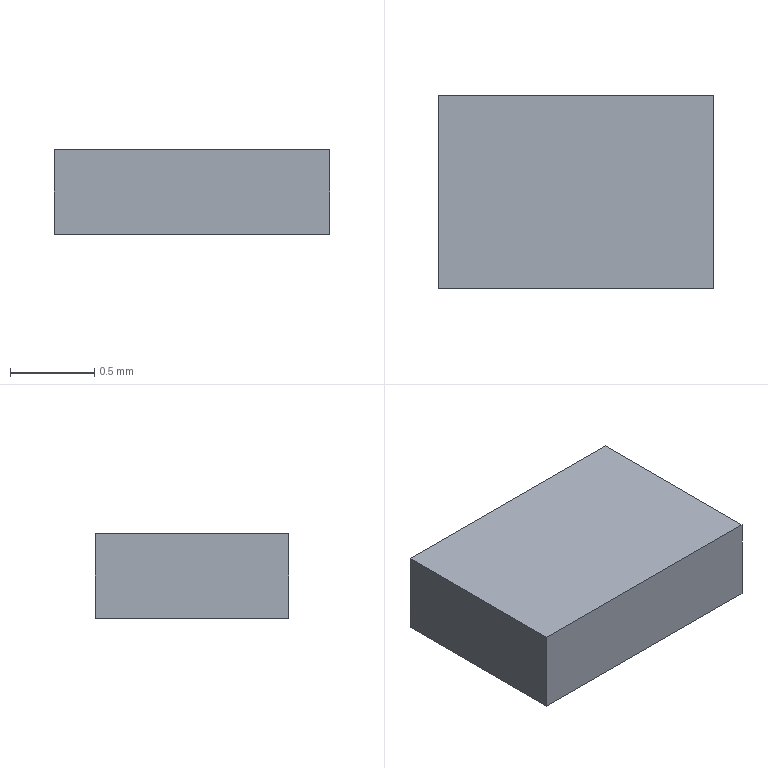Part | Creo | 1 solid | 6 faces | box 1.64 x 1.15 x 0.5 mm | volume 0.9427 mm3 | plane 6
STEP:
#1=CARTESIAN_POINT('',(0.,0.,0.));
#2=DIRECTION('',(0.,0.,1.));
#3=DIRECTION('',(1.,0.,0.));
#4=AXIS2_PLACEMENT_3D('',#1,#2,#3);
#5=CARTESIAN_POINT('',(-0.9145,-0.575,0.));
#6=VERTEX_POINT('',#5);
#7=CARTESIAN_POINT('',(0.725,-0.575,0.));
#8=VERTEX_POINT('',#7);
#9=CARTESIAN_POINT('',(-0.9145,-0.575,0.));
#10=DIRECTION('',(1.,0.,0.));
#11=VECTOR('',#10,1.64);
#12=LINE('',#9,#11);
#13=EDGE_CURVE('',#6,#8,#12,.T.);
#14=ORIENTED_EDGE('',*,*,#13,.T.);
#15=CARTESIAN_POINT('',(0.725,0.575,0.));
#16=VERTEX_POINT('',#15);
#17=CARTESIAN_POINT('',(0.725,-0.575,0.));
#18=DIRECTION('',(0.,1.,0.));
#19=VECTOR('',#18,1.15);
#20=LINE('',#17,#19);
#21=EDGE_CURVE('',#8,#16,#20,.T.);
#22=ORIENTED_EDGE('',*,*,#21,.T.);
#23=CARTESIAN_POINT('',(-0.9145,0.575,0.));
#24=VERTEX_POINT('',#23);
#25=CARTESIAN_POINT('',(0.725,0.575,0.));
#26=DIRECTION('',(-1.,0.,0.));
#27=VECTOR('',#26,1.64);
#28=LINE('',#25,#27);
#29=EDGE_CURVE('',#16,#24,#28,.T.);
#30=ORIENTED_EDGE('',*,*,#29,.T.);
#31=CARTESIAN_POINT('',(-0.9145,0.575,0.));
#32=DIRECTION('',(0.,-1.,0.));
#33=VECTOR('',#32,1.15);
#34=LINE('',#31,#33);
#35=EDGE_CURVE('',#24,#6,#34,.T.);
#36=ORIENTED_EDGE('',*,*,#35,.T.);
#37=EDGE_LOOP('',(#14,#22,#30,#36));
#38=FACE_OUTER_BOUND('',#37,.F.);
#39=CARTESIAN_POINT('',(0.,0.,0.));
#40=DIRECTION('',(0.,0.,1.));
#41=DIRECTION('',(1.,0.,0.));
#42=AXIS2_PLACEMENT_3D('',#39,#40,#41);
#43=PLANE('',#42);
#44=ADVANCED_FACE('',(#38),#43,.F.);
#45=ORIENTED_EDGE('',*,*,#13,.F.);
#46=CARTESIAN_POINT('',(-0.9145,-0.575,0.5));
#47=VERTEX_POINT('',#46);
#48=CARTESIAN_POINT('',(-0.9145,-0.575,0.));
#49=DIRECTION('',(0.,0.,1.));
#50=VECTOR('',#49,0.5);
#51=LINE('',#48,#50);
#52=EDGE_CURVE('',#6,#47,#51,.T.);
#53=ORIENTED_EDGE('',*,*,#52,.T.);
#54=CARTESIAN_POINT('',(0.725,-0.575,0.5));
#55=VERTEX_POINT('',#54);
#56=CARTESIAN_POINT('',(-0.9145,-0.575,0.5));
#57=DIRECTION('',(1.,0.,0.));
#58=VECTOR('',#57,1.64);
#59=LINE('',#56,#58);
#60=EDGE_CURVE('',#47,#55,#59,.T.);
#61=ORIENTED_EDGE('',*,*,#60,.T.);
#62=CARTESIAN_POINT('',(0.725,-0.575,0.));
#63=DIRECTION('',(0.,0.,1.));
#64=VECTOR('',#63,0.5);
#65=LINE('',#62,#64);
#66=EDGE_CURVE('',#8,#55,#65,.T.);
#67=ORIENTED_EDGE('',*,*,#66,.F.);
#68=EDGE_LOOP('',(#45,#53,#61,#67));
#69=FACE_OUTER_BOUND('',#68,.F.);
#70=CARTESIAN_POINT('',(-0.9145,-0.575,0.));
#71=DIRECTION('',(0.,-1.,0.));
#72=DIRECTION('',(1.,0.,0.));
#73=AXIS2_PLACEMENT_3D('',#70,#71,#72);
#74=PLANE('',#73);
#75=ADVANCED_FACE('',(#69),#74,.T.);
#76=ORIENTED_EDGE('',*,*,#35,.F.);
#77=CARTESIAN_POINT('',(-0.9145,0.575,0.5));
#78=VERTEX_POINT('',#77);
#79=CARTESIAN_POINT('',(-0.9145,0.575,0.));
#80=DIRECTION('',(0.,0.,1.));
#81=VECTOR('',#80,0.5);
#82=LINE('',#79,#81);
#83=EDGE_CURVE('',#24,#78,#82,.T.);
#84=ORIENTED_EDGE('',*,*,#83,.T.);
#85=CARTESIAN_POINT('',(-0.9145,0.575,0.5));
#86=DIRECTION('',(0.,-1.,0.));
#87=VECTOR('',#86,1.15);
#88=LINE('',#85,#87);
#89=EDGE_CURVE('',#78,#47,#88,.T.);
#90=ORIENTED_EDGE('',*,*,#89,.T.);
#91=ORIENTED_EDGE('',*,*,#52,.F.);
#92=EDGE_LOOP('',(#76,#84,#90,#91));
#93=FACE_OUTER_BOUND('',#92,.F.);
#94=CARTESIAN_POINT('',(-0.9145,0.575,0.));
#95=DIRECTION('',(-1.,0.,0.));
#96=DIRECTION('',(0.,-1.,0.));
#97=AXIS2_PLACEMENT_3D('',#94,#95,#96);
#98=PLANE('',#97);
#99=ADVANCED_FACE('',(#93),#98,.T.);
#100=ORIENTED_EDGE('',*,*,#29,.F.);
#101=CARTESIAN_POINT('',(0.725,0.575,0.5));
#102=VERTEX_POINT('',#101);
#103=CARTESIAN_POINT('',(0.725,0.575,0.));
#104=DIRECTION('',(0.,0.,1.));
#105=VECTOR('',#104,0.5);
#106=LINE('',#103,#105);
#107=EDGE_CURVE('',#16,#102,#106,.T.);
#108=ORIENTED_EDGE('',*,*,#107,.T.);
#109=CARTESIAN_POINT('',(0.725,0.575,0.5));
#110=DIRECTION('',(-1.,0.,0.));
#111=VECTOR('',#110,1.64);
#112=LINE('',#109,#111);
#113=EDGE_CURVE('',#102,#78,#112,.T.);
#114=ORIENTED_EDGE('',*,*,#113,.T.);
#115=ORIENTED_EDGE('',*,*,#83,.F.);
#116=EDGE_LOOP('',(#100,#108,#114,#115));
#117=FACE_OUTER_BOUND('',#116,.F.);
#118=CARTESIAN_POINT('',(0.725,0.575,0.));
#119=DIRECTION('',(0.,1.,0.));
#120=DIRECTION('',(-1.,0.,0.));
#121=AXIS2_PLACEMENT_3D('',#118,#119,#120);
#122=PLANE('',#121);
#123=ADVANCED_FACE('',(#117),#122,.T.);
#124=ORIENTED_EDGE('',*,*,#21,.F.);
#125=ORIENTED_EDGE('',*,*,#66,.T.);
#126=CARTESIAN_POINT('',(0.725,-0.575,0.5));
#127=DIRECTION('',(0.,1.,0.));
#128=VECTOR('',#127,1.15);
#129=LINE('',#126,#128);
#130=EDGE_CURVE('',#55,#102,#129,.T.);
#131=ORIENTED_EDGE('',*,*,#130,.T.);
#132=ORIENTED_EDGE('',*,*,#107,.F.);
#133=EDGE_LOOP('',(#124,#125,#131,#132));
#134=FACE_OUTER_BOUND('',#133,.F.);
#135=CARTESIAN_POINT('',(0.725,-0.575,0.));
#136=DIRECTION('',(1.,0.,0.));
#137=DIRECTION('',(0.,1.,0.));
#138=AXIS2_PLACEMENT_3D('',#135,#136,#137);
#139=PLANE('',#138);
#140=ADVANCED_FACE('',(#134),#139,.T.);
#141=ORIENTED_EDGE('',*,*,#60,.F.);
#142=ORIENTED_EDGE('',*,*,#89,.F.);
#143=ORIENTED_EDGE('',*,*,#113,.F.);
#144=ORIENTED_EDGE('',*,*,#130,.F.);
#145=EDGE_LOOP('',(#141,#142,#143,#144));
#146=FACE_OUTER_BOUND('',#145,.F.);
#147=CARTESIAN_POINT('',(0.,0.,0.5));
#148=DIRECTION('',(0.,0.,1.));
#149=DIRECTION('',(1.,0.,0.));
#150=AXIS2_PLACEMENT_3D('',#147,#148,#149);
#151=PLANE('',#150);
#152=ADVANCED_FACE('',(#146),#151,.T.);
#153=CLOSED_SHELL('',(#44,#75,#99,#123,#140,#152));
#154=MANIFOLD_SOLID_BREP('',#153);
#155=(LENGTH_UNIT()NAMED_UNIT(*)SI_UNIT(.MILLI.,.METRE.));
#156=UNCERTAINTY_MEASURE_WITH_UNIT(LENGTH_MEASURE(0.0002064),#155,'','');
#157=(NAMED_UNIT(*)PLANE_ANGLE_UNIT()SI_UNIT($,.RADIAN.));
#158=PLANE_ANGLE_MEASURE_WITH_UNIT(PLANE_ANGLE_MEASURE(0.01745),#157);
#159=(CONVERSION_BASED_UNIT('DEGREE',#158)NAMED_UNIT(*)PLANE_ANGLE_UNIT());
#160=(NAMED_UNIT(*)SI_UNIT($,.STERADIAN.)SOLID_ANGLE_UNIT());
#161=(GEOMETRIC_REPRESENTATION_CONTEXT(3)GLOBAL_UNCERTAINTY_ASSIGNED_CONTEXT((#156))GLOBAL_UNIT_ASSIGNED_CONTEXT((#155,#159,#160))REPRESENTATION_CONTEXT('',''));
#162=ADVANCED_BREP_SHAPE_REPRESENTATION('',(#4,#154),#161);